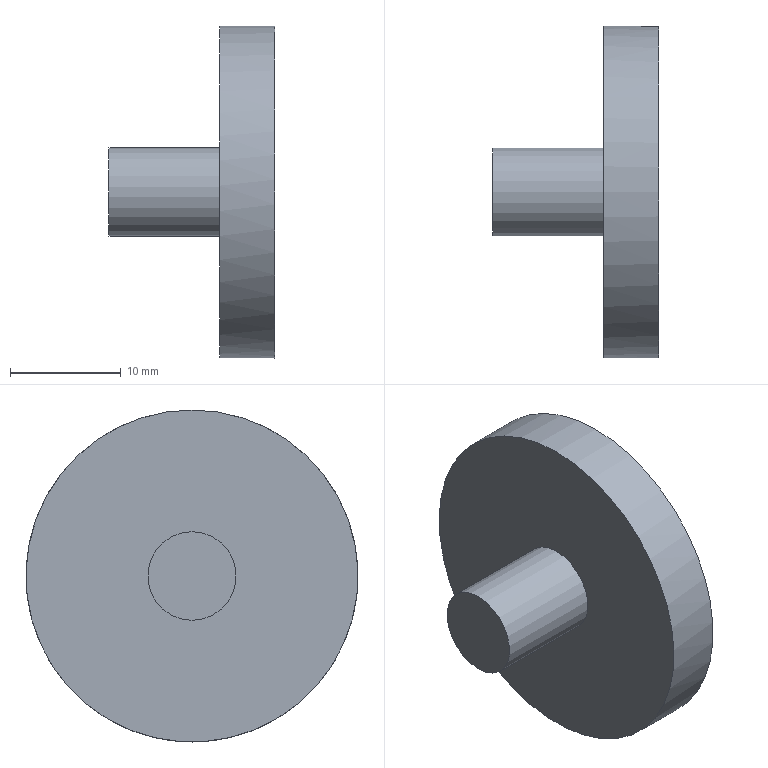Part | STEP file | solid 62 | 1 solid | 5 faces | box 15 x 30 x 30 mm | volume 4037 mm3 | plane 3 | cylinder 2 | commonest cylinder face diameters 8 x1 30 x1